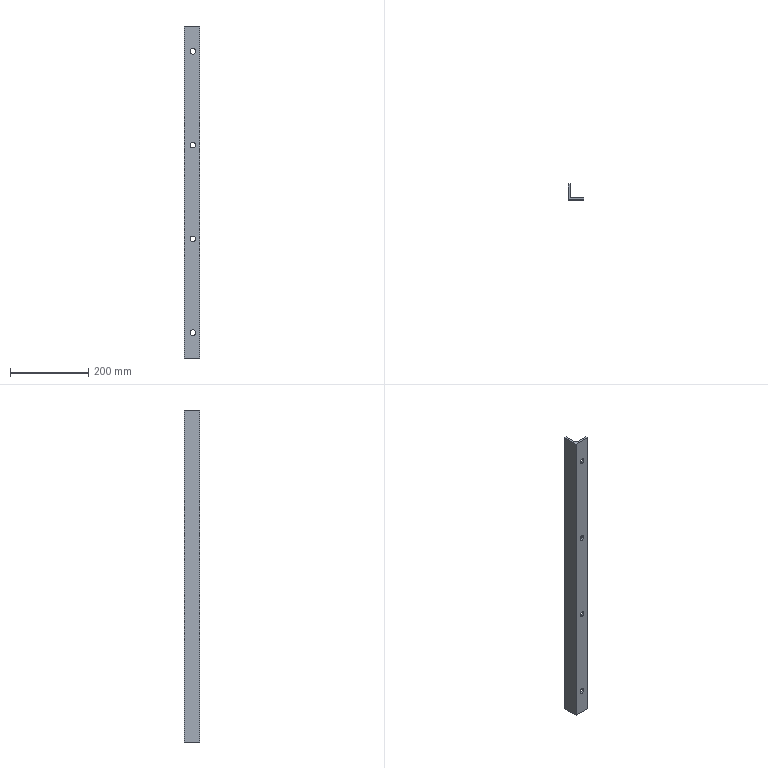Part | NX | features BREP 1 | 1 solid | 17 faces | box 40 x 40 x 850 mm | volume 320232 mm3 | cylinder 9 | plane 8 | commonest cylinder face diameters 14 x8 10 x1
STEP:
#1=CARTESIAN_POINT('',(22.,0.,353.));
#2=VERTEX_POINT('',#1);
#3=CARTESIAN_POINT('',(22.,0.,367.));
#4=VERTEX_POINT('',#3);
#5=CARTESIAN_POINT('',(22.,0.,360.));
#6=DIRECTION('',(0.,1.,0.));
#7=DIRECTION('',(0.,0.,-1.));
#8=AXIS2_PLACEMENT_3D('',#5,#6,#7);
#9=CIRCLE('',#8,7.);
#10=EDGE_CURVE('',#2,#4,#9,.T.);
#11=ORIENTED_EDGE('',*,*,#10,.F.);
#12=CARTESIAN_POINT('',(22.,5.,353.));
#13=VERTEX_POINT('',#12);
#14=CARTESIAN_POINT('',(22.,0.,353.));
#15=DIRECTION('',(0.,1.,0.));
#16=VECTOR('',#15,1000.);
#17=LINE('',#14,#16);
#18=EDGE_CURVE('',#2,#13,#17,.T.);
#19=ORIENTED_EDGE('',*,*,#18,.T.);
#20=CARTESIAN_POINT('',(22.,5.,367.));
#21=VERTEX_POINT('',#20);
#22=CARTESIAN_POINT('',(22.,5.,360.));
#23=DIRECTION('',(0.,1.,0.));
#24=DIRECTION('',(0.,0.,-1.));
#25=AXIS2_PLACEMENT_3D('',#22,#23,#24);
#26=CIRCLE('',#25,7.);
#27=EDGE_CURVE('',#13,#21,#26,.T.);
#28=ORIENTED_EDGE('',*,*,#27,.T.);
#29=CARTESIAN_POINT('',(22.,0.,367.));
#30=DIRECTION('',(0.,1.,0.));
#31=VECTOR('',#30,1000.);
#32=LINE('',#29,#31);
#33=EDGE_CURVE('',#4,#21,#32,.T.);
#34=ORIENTED_EDGE('',*,*,#33,.F.);
#35=EDGE_LOOP('',(#11,#19,#28,#34));
#36=FACE_BOUND('',#35,.T.);
#37=CARTESIAN_POINT('',(22.,0.,360.));
#38=DIRECTION('',(0.,1.,0.));
#39=DIRECTION('',(0.,0.,-1.));
#40=AXIS2_PLACEMENT_3D('',#37,#38,#39);
#41=CYLINDRICAL_SURFACE('',#40,7.);
#42=ADVANCED_FACE('',(#36),#41,.F.);
#43=CARTESIAN_POINT('',(22.,0.,113.));
#44=VERTEX_POINT('',#43);
#45=CARTESIAN_POINT('',(22.,0.,127.));
#46=VERTEX_POINT('',#45);
#47=CARTESIAN_POINT('',(22.,0.,120.));
#48=DIRECTION('',(0.,1.,0.));
#49=DIRECTION('',(0.,0.,-1.));
#50=AXIS2_PLACEMENT_3D('',#47,#48,#49);
#51=CIRCLE('',#50,7.);
#52=EDGE_CURVE('',#44,#46,#51,.T.);
#53=ORIENTED_EDGE('',*,*,#52,.F.);
#54=CARTESIAN_POINT('',(22.,5.,113.));
#55=VERTEX_POINT('',#54);
#56=CARTESIAN_POINT('',(22.,0.,113.));
#57=DIRECTION('',(0.,1.,0.));
#58=VECTOR('',#57,1000.);
#59=LINE('',#56,#58);
#60=EDGE_CURVE('',#44,#55,#59,.T.);
#61=ORIENTED_EDGE('',*,*,#60,.T.);
#62=CARTESIAN_POINT('',(22.,5.,127.));
#63=VERTEX_POINT('',#62);
#64=CARTESIAN_POINT('',(22.,5.,120.));
#65=DIRECTION('',(0.,1.,0.));
#66=DIRECTION('',(0.,0.,-1.));
#67=AXIS2_PLACEMENT_3D('',#64,#65,#66);
#68=CIRCLE('',#67,7.);
#69=EDGE_CURVE('',#55,#63,#68,.T.);
#70=ORIENTED_EDGE('',*,*,#69,.T.);
#71=CARTESIAN_POINT('',(22.,0.,127.));
#72=DIRECTION('',(0.,1.,0.));
#73=VECTOR('',#72,1000.);
#74=LINE('',#71,#73);
#75=EDGE_CURVE('',#46,#63,#74,.T.);
#76=ORIENTED_EDGE('',*,*,#75,.F.);
#77=EDGE_LOOP('',(#53,#61,#70,#76));
#78=FACE_BOUND('',#77,.T.);
#79=CARTESIAN_POINT('',(22.,0.,120.));
#80=DIRECTION('',(0.,1.,0.));
#81=DIRECTION('',(0.,0.,-1.));
#82=AXIS2_PLACEMENT_3D('',#79,#80,#81);
#83=CYLINDRICAL_SURFACE('',#82,7.);
#84=ADVANCED_FACE('',(#78),#83,.F.);
#85=CARTESIAN_POINT('',(22.,0.,-127.));
#86=VERTEX_POINT('',#85);
#87=CARTESIAN_POINT('',(22.,0.,-113.));
#88=VERTEX_POINT('',#87);
#89=CARTESIAN_POINT('',(22.,0.,-120.));
#90=DIRECTION('',(0.,1.,0.));
#91=DIRECTION('',(0.,0.,1.));
#92=AXIS2_PLACEMENT_3D('',#89,#90,#91);
#93=CIRCLE('',#92,7.);
#94=EDGE_CURVE('',#86,#88,#93,.T.);
#95=ORIENTED_EDGE('',*,*,#94,.F.);
#96=CARTESIAN_POINT('',(22.,5.,-127.));
#97=VERTEX_POINT('',#96);
#98=CARTESIAN_POINT('',(22.,0.,-127.));
#99=DIRECTION('',(0.,1.,0.));
#100=VECTOR('',#99,1000.);
#101=LINE('',#98,#100);
#102=EDGE_CURVE('',#86,#97,#101,.T.);
#103=ORIENTED_EDGE('',*,*,#102,.T.);
#104=CARTESIAN_POINT('',(22.,5.,-113.));
#105=VERTEX_POINT('',#104);
#106=CARTESIAN_POINT('',(22.,5.,-120.));
#107=DIRECTION('',(0.,1.,0.));
#108=DIRECTION('',(0.,0.,1.));
#109=AXIS2_PLACEMENT_3D('',#106,#107,#108);
#110=CIRCLE('',#109,7.);
#111=EDGE_CURVE('',#97,#105,#110,.T.);
#112=ORIENTED_EDGE('',*,*,#111,.T.);
#113=CARTESIAN_POINT('',(22.,0.,-113.));
#114=DIRECTION('',(0.,1.,0.));
#115=VECTOR('',#114,1000.);
#116=LINE('',#113,#115);
#117=EDGE_CURVE('',#88,#105,#116,.T.);
#118=ORIENTED_EDGE('',*,*,#117,.F.);
#119=EDGE_LOOP('',(#95,#103,#112,#118));
#120=FACE_BOUND('',#119,.T.);
#121=CARTESIAN_POINT('',(22.,0.,-120.));
#122=DIRECTION('',(0.,1.,0.));
#123=DIRECTION('',(0.,0.,-1.));
#124=AXIS2_PLACEMENT_3D('',#121,#122,#123);
#125=CYLINDRICAL_SURFACE('',#124,7.);
#126=ADVANCED_FACE('',(#120),#125,.F.);
#127=CARTESIAN_POINT('',(22.,0.,-367.));
#128=VERTEX_POINT('',#127);
#129=CARTESIAN_POINT('',(22.,0.,-353.));
#130=VERTEX_POINT('',#129);
#131=CARTESIAN_POINT('',(22.,0.,-360.));
#132=DIRECTION('',(0.,1.,0.));
#133=DIRECTION('',(0.,0.,1.));
#134=AXIS2_PLACEMENT_3D('',#131,#132,#133);
#135=CIRCLE('',#134,7.);
#136=EDGE_CURVE('',#128,#130,#135,.T.);
#137=ORIENTED_EDGE('',*,*,#136,.F.);
#138=CARTESIAN_POINT('',(22.,5.,-367.));
#139=VERTEX_POINT('',#138);
#140=CARTESIAN_POINT('',(22.,0.,-367.));
#141=DIRECTION('',(0.,1.,0.));
#142=VECTOR('',#141,1000.);
#143=LINE('',#140,#142);
#144=EDGE_CURVE('',#128,#139,#143,.T.);
#145=ORIENTED_EDGE('',*,*,#144,.T.);
#146=CARTESIAN_POINT('',(22.,5.,-353.));
#147=VERTEX_POINT('',#146);
#148=CARTESIAN_POINT('',(22.,5.,-360.));
#149=DIRECTION('',(0.,1.,0.));
#150=DIRECTION('',(0.,0.,1.));
#151=AXIS2_PLACEMENT_3D('',#148,#149,#150);
#152=CIRCLE('',#151,7.);
#153=EDGE_CURVE('',#139,#147,#152,.T.);
#154=ORIENTED_EDGE('',*,*,#153,.T.);
#155=CARTESIAN_POINT('',(22.,0.,-353.));
#156=DIRECTION('',(0.,1.,0.));
#157=VECTOR('',#156,1000.);
#158=LINE('',#155,#157);
#159=EDGE_CURVE('',#130,#147,#158,.T.);
#160=ORIENTED_EDGE('',*,*,#159,.F.);
#161=EDGE_LOOP('',(#137,#145,#154,#160));
#162=FACE_BOUND('',#161,.T.);
#163=CARTESIAN_POINT('',(22.,0.,-360.));
#164=DIRECTION('',(0.,1.,0.));
#165=DIRECTION('',(0.,0.,-1.));
#166=AXIS2_PLACEMENT_3D('',#163,#164,#165);
#167=CYLINDRICAL_SURFACE('',#166,7.);
#168=ADVANCED_FACE('',(#162),#167,.F.);
#169=CARTESIAN_POINT('',(40.,0.,-425.));
#170=VERTEX_POINT('',#169);
#171=CARTESIAN_POINT('',(40.,5.,-425.));
#172=VERTEX_POINT('',#171);
#173=CARTESIAN_POINT('',(40.,5.,-425.));
#174=DIRECTION('',(0.,1.,0.));
#175=VECTOR('',#174,1000.);
#176=LINE('',#173,#175);
#177=EDGE_CURVE('',#170,#172,#176,.T.);
#178=ORIENTED_EDGE('',*,*,#177,.T.);
#179=CARTESIAN_POINT('',(40.,5.,425.));
#180=VERTEX_POINT('',#179);
#181=CARTESIAN_POINT('',(40.,5.,425.));
#182=DIRECTION('',(0.,0.,-1.));
#183=VECTOR('',#182,1000.);
#184=LINE('',#181,#183);
#185=EDGE_CURVE('',#180,#172,#184,.T.);
#186=ORIENTED_EDGE('',*,*,#185,.F.);
#187=CARTESIAN_POINT('',(40.,0.,425.));
#188=VERTEX_POINT('',#187);
#189=CARTESIAN_POINT('',(40.,5.,425.));
#190=DIRECTION('',(0.,1.,0.));
#191=VECTOR('',#190,1000.);
#192=LINE('',#189,#191);
#193=EDGE_CURVE('',#188,#180,#192,.T.);
#194=ORIENTED_EDGE('',*,*,#193,.F.);
#195=CARTESIAN_POINT('',(40.,0.,425.));
#196=DIRECTION('',(0.,0.,-1.));
#197=VECTOR('',#196,1000.);
#198=LINE('',#195,#197);
#199=EDGE_CURVE('',#188,#170,#198,.T.);
#200=ORIENTED_EDGE('',*,*,#199,.T.);
#201=EDGE_LOOP('',(#178,#186,#194,#200));
#202=FACE_BOUND('',#201,.T.);
#203=CARTESIAN_POINT('',(40.,5.,425.));
#204=DIRECTION('',(-1.,0.,0.));
#205=DIRECTION('',(0.,0.,-1.));
#206=AXIS2_PLACEMENT_3D('',#203,#204,#205);
#207=PLANE('',#206);
#208=ADVANCED_FACE('',(#202),#207,.F.);
#209=CARTESIAN_POINT('',(22.,5.,360.));
#210=DIRECTION('',(0.,1.,0.));
#211=DIRECTION('',(0.,0.,-1.));
#212=AXIS2_PLACEMENT_3D('',#209,#210,#211);
#213=CIRCLE('',#212,7.);
#214=EDGE_CURVE('',#21,#13,#213,.T.);
#215=ORIENTED_EDGE('',*,*,#214,.F.);
#216=ORIENTED_EDGE('',*,*,#27,.F.);
#217=EDGE_LOOP('',(#215,#216));
#218=FACE_BOUND('',#217,.T.);
#219=CARTESIAN_POINT('',(22.,5.,120.));
#220=DIRECTION('',(0.,1.,0.));
#221=DIRECTION('',(0.,0.,-1.));
#222=AXIS2_PLACEMENT_3D('',#219,#220,#221);
#223=CIRCLE('',#222,7.);
#224=EDGE_CURVE('',#63,#55,#223,.T.);
#225=ORIENTED_EDGE('',*,*,#224,.F.);
#226=ORIENTED_EDGE('',*,*,#69,.F.);
#227=EDGE_LOOP('',(#225,#226));
#228=FACE_BOUND('',#227,.T.);
#229=CARTESIAN_POINT('',(22.,5.,-120.));
#230=DIRECTION('',(0.,1.,0.));
#231=DIRECTION('',(0.,0.,1.));
#232=AXIS2_PLACEMENT_3D('',#229,#230,#231);
#233=CIRCLE('',#232,7.);
#234=EDGE_CURVE('',#105,#97,#233,.T.);
#235=ORIENTED_EDGE('',*,*,#234,.F.);
#236=ORIENTED_EDGE('',*,*,#111,.F.);
#237=EDGE_LOOP('',(#235,#236));
#238=FACE_BOUND('',#237,.T.);
#239=CARTESIAN_POINT('',(22.,5.,-360.));
#240=DIRECTION('',(0.,1.,0.));
#241=DIRECTION('',(0.,0.,1.));
#242=AXIS2_PLACEMENT_3D('',#239,#240,#241);
#243=CIRCLE('',#242,7.);
#244=EDGE_CURVE('',#147,#139,#243,.T.);
#245=ORIENTED_EDGE('',*,*,#244,.F.);
#246=ORIENTED_EDGE('',*,*,#153,.F.);
#247=EDGE_LOOP('',(#245,#246));
#248=FACE_BOUND('',#247,.T.);
#249=CARTESIAN_POINT('',(10.,5.,-425.));
#250=VERTEX_POINT('',#249);
#251=CARTESIAN_POINT('',(10.,5.,-425.));
#252=DIRECTION('',(-1.,0.,0.));
#253=VECTOR('',#252,1000.);
#254=LINE('',#251,#253);
#255=EDGE_CURVE('',#172,#250,#254,.T.);
#256=ORIENTED_EDGE('',*,*,#255,.T.);
#257=CARTESIAN_POINT('',(10.,5.,425.));
#258=VERTEX_POINT('',#257);
#259=CARTESIAN_POINT('',(10.,5.,425.));
#260=DIRECTION('',(0.,0.,-1.));
#261=VECTOR('',#260,1000.);
#262=LINE('',#259,#261);
#263=EDGE_CURVE('',#258,#250,#262,.T.);
#264=ORIENTED_EDGE('',*,*,#263,.F.);
#265=CARTESIAN_POINT('',(10.,5.,425.));
#266=DIRECTION('',(-1.,0.,0.));
#267=VECTOR('',#266,1000.);
#268=LINE('',#265,#267);
#269=EDGE_CURVE('',#180,#258,#268,.T.);
#270=ORIENTED_EDGE('',*,*,#269,.F.);
#271=ORIENTED_EDGE('',*,*,#185,.T.);
#272=EDGE_LOOP('',(#256,#264,#270,#271));
#273=FACE_BOUND('',#272,.T.);
#274=CARTESIAN_POINT('',(10.,5.,425.));
#275=DIRECTION('',(0.,-1.,0.));
#276=DIRECTION('',(0.,0.,1.));
#277=AXIS2_PLACEMENT_3D('',#274,#275,#276);
#278=PLANE('',#277);
#279=ADVANCED_FACE('',(#218,#228,#238,#248,#273),#278,.F.);
#280=CARTESIAN_POINT('',(5.,10.,-425.));
#281=VERTEX_POINT('',#280);
#282=CARTESIAN_POINT('',(10.,10.,-425.));
#283=DIRECTION('',(0.,0.,-1.));
#284=DIRECTION('',(1.,0.,0.));
#285=AXIS2_PLACEMENT_3D('',#282,#283,#284);
#286=CIRCLE('',#285,5.);
#287=EDGE_CURVE('',#250,#281,#286,.T.);
#288=ORIENTED_EDGE('',*,*,#287,.T.);
#289=CARTESIAN_POINT('',(5.,10.,425.));
#290=VERTEX_POINT('',#289);
#291=CARTESIAN_POINT('',(5.,10.,425.));
#292=DIRECTION('',(0.,0.,-1.));
#293=VECTOR('',#292,1000.);
#294=LINE('',#291,#293);
#295=EDGE_CURVE('',#290,#281,#294,.T.);
#296=ORIENTED_EDGE('',*,*,#295,.F.);
#297=CARTESIAN_POINT('',(10.,10.,425.));
#298=DIRECTION('',(0.,0.,-1.));
#299=DIRECTION('',(1.,0.,0.));
#300=AXIS2_PLACEMENT_3D('',#297,#298,#299);
#301=CIRCLE('',#300,5.);
#302=EDGE_CURVE('',#258,#290,#301,.T.);
#303=ORIENTED_EDGE('',*,*,#302,.F.);
#304=ORIENTED_EDGE('',*,*,#263,.T.);
#305=EDGE_LOOP('',(#288,#296,#303,#304));
#306=FACE_BOUND('',#305,.T.);
#307=CARTESIAN_POINT('',(10.,10.,425.));
#308=DIRECTION('',(0.,0.,-1.));
#309=DIRECTION('',(1.,0.,0.));
#310=AXIS2_PLACEMENT_3D('',#307,#308,#309);
#311=CYLINDRICAL_SURFACE('',#310,5.);
#312=ADVANCED_FACE('',(#306),#311,.F.);
#313=CARTESIAN_POINT('',(5.,40.,-425.));
#314=VERTEX_POINT('',#313);
#315=CARTESIAN_POINT('',(5.,40.,-425.));
#316=DIRECTION('',(0.,1.,0.));
#317=VECTOR('',#316,1000.);
#318=LINE('',#315,#317);
#319=EDGE_CURVE('',#281,#314,#318,.T.);
#320=ORIENTED_EDGE('',*,*,#319,.T.);
#321=CARTESIAN_POINT('',(5.,40.,425.));
#322=VERTEX_POINT('',#321);
#323=CARTESIAN_POINT('',(5.,40.,425.));
#324=DIRECTION('',(0.,0.,-1.));
#325=VECTOR('',#324,1000.);
#326=LINE('',#323,#325);
#327=EDGE_CURVE('',#322,#314,#326,.T.);
#328=ORIENTED_EDGE('',*,*,#327,.F.);
#329=CARTESIAN_POINT('',(5.,40.,425.));
#330=DIRECTION('',(0.,1.,0.));
#331=VECTOR('',#330,1000.);
#332=LINE('',#329,#331);
#333=EDGE_CURVE('',#290,#322,#332,.T.);
#334=ORIENTED_EDGE('',*,*,#333,.F.);
#335=ORIENTED_EDGE('',*,*,#295,.T.);
#336=EDGE_LOOP('',(#320,#328,#334,#335));
#337=FACE_BOUND('',#336,.T.);
#338=CARTESIAN_POINT('',(5.,40.,425.));
#339=DIRECTION('',(-1.,0.,0.));
#340=DIRECTION('',(0.,0.,-1.));
#341=AXIS2_PLACEMENT_3D('',#338,#339,#340);
#342=PLANE('',#341);
#343=ADVANCED_FACE('',(#337),#342,.F.);
#344=CARTESIAN_POINT('',(0.,40.,-425.));
#345=VERTEX_POINT('',#344);
#346=CARTESIAN_POINT('',(0.,40.,-425.));
#347=DIRECTION('',(-1.,0.,0.));
#348=VECTOR('',#347,1000.);
#349=LINE('',#346,#348);
#350=EDGE_CURVE('',#314,#345,#349,.T.);
#351=ORIENTED_EDGE('',*,*,#350,.T.);
#352=CARTESIAN_POINT('',(0.,40.,425.));
#353=VERTEX_POINT('',#352);
#354=CARTESIAN_POINT('',(0.,40.,425.));
#355=DIRECTION('',(0.,0.,-1.));
#356=VECTOR('',#355,1000.);
#357=LINE('',#354,#356);
#358=EDGE_CURVE('',#353,#345,#357,.T.);
#359=ORIENTED_EDGE('',*,*,#358,.F.);
#360=CARTESIAN_POINT('',(0.,40.,425.));
#361=DIRECTION('',(-1.,0.,0.));
#362=VECTOR('',#361,1000.);
#363=LINE('',#360,#362);
#364=EDGE_CURVE('',#322,#353,#363,.T.);
#365=ORIENTED_EDGE('',*,*,#364,.F.);
#366=ORIENTED_EDGE('',*,*,#327,.T.);
#367=EDGE_LOOP('',(#351,#359,#365,#366));
#368=FACE_BOUND('',#367,.T.);
#369=CARTESIAN_POINT('',(0.,40.,425.));
#370=DIRECTION('',(0.,-1.,0.));
#371=DIRECTION('',(0.,0.,1.));
#372=AXIS2_PLACEMENT_3D('',#369,#370,#371);
#373=PLANE('',#372);
#374=ADVANCED_FACE('',(#368),#373,.F.);
#375=CARTESIAN_POINT('',(0.,0.,-425.));
#376=VERTEX_POINT('',#375);
#377=CARTESIAN_POINT('',(0.,0.,-425.));
#378=DIRECTION('',(0.,-1.,0.));
#379=VECTOR('',#378,1000.);
#380=LINE('',#377,#379);
#381=EDGE_CURVE('',#345,#376,#380,.T.);
#382=ORIENTED_EDGE('',*,*,#381,.T.);
#383=CARTESIAN_POINT('',(0.,0.,425.));
#384=VERTEX_POINT('',#383);
#385=CARTESIAN_POINT('',(0.,0.,425.));
#386=DIRECTION('',(0.,0.,-1.));
#387=VECTOR('',#386,1000.);
#388=LINE('',#385,#387);
#389=EDGE_CURVE('',#384,#376,#388,.T.);
#390=ORIENTED_EDGE('',*,*,#389,.F.);
#391=CARTESIAN_POINT('',(0.,0.,425.));
#392=DIRECTION('',(0.,-1.,0.));
#393=VECTOR('',#392,1000.);
#394=LINE('',#391,#393);
#395=EDGE_CURVE('',#353,#384,#394,.T.);
#396=ORIENTED_EDGE('',*,*,#395,.F.);
#397=ORIENTED_EDGE('',*,*,#358,.T.);
#398=EDGE_LOOP('',(#382,#390,#396,#397));
#399=FACE_BOUND('',#398,.T.);
#400=CARTESIAN_POINT('',(0.,0.,425.));
#401=DIRECTION('',(1.,0.,0.));
#402=DIRECTION('',(0.,0.,1.));
#403=AXIS2_PLACEMENT_3D('',#400,#401,#402);
#404=PLANE('',#403);
#405=ADVANCED_FACE('',(#399),#404,.F.);
#406=CARTESIAN_POINT('',(22.,0.,360.));
#407=DIRECTION('',(0.,1.,0.));
#408=DIRECTION('',(0.,0.,-1.));
#409=AXIS2_PLACEMENT_3D('',#406,#407,#408);
#410=CIRCLE('',#409,7.);
#411=EDGE_CURVE('',#4,#2,#410,.T.);
#412=ORIENTED_EDGE('',*,*,#411,.T.);
#413=ORIENTED_EDGE('',*,*,#10,.T.);
#414=EDGE_LOOP('',(#412,#413));
#415=FACE_BOUND('',#414,.T.);
#416=CARTESIAN_POINT('',(22.,0.,120.));
#417=DIRECTION('',(0.,1.,0.));
#418=DIRECTION('',(0.,0.,-1.));
#419=AXIS2_PLACEMENT_3D('',#416,#417,#418);
#420=CIRCLE('',#419,7.);
#421=EDGE_CURVE('',#46,#44,#420,.T.);
#422=ORIENTED_EDGE('',*,*,#421,.T.);
#423=ORIENTED_EDGE('',*,*,#52,.T.);
#424=EDGE_LOOP('',(#422,#423));
#425=FACE_BOUND('',#424,.T.);
#426=CARTESIAN_POINT('',(22.,0.,-120.));
#427=DIRECTION('',(0.,1.,0.));
#428=DIRECTION('',(0.,0.,1.));
#429=AXIS2_PLACEMENT_3D('',#426,#427,#428);
#430=CIRCLE('',#429,7.);
#431=EDGE_CURVE('',#88,#86,#430,.T.);
#432=ORIENTED_EDGE('',*,*,#431,.T.);
#433=ORIENTED_EDGE('',*,*,#94,.T.);
#434=EDGE_LOOP('',(#432,#433));
#435=FACE_BOUND('',#434,.T.);
#436=CARTESIAN_POINT('',(22.,0.,-360.));
#437=DIRECTION('',(0.,1.,0.));
#438=DIRECTION('',(0.,0.,1.));
#439=AXIS2_PLACEMENT_3D('',#436,#437,#438);
#440=CIRCLE('',#439,7.);
#441=EDGE_CURVE('',#130,#128,#440,.T.);
#442=ORIENTED_EDGE('',*,*,#441,.T.);
#443=ORIENTED_EDGE('',*,*,#136,.T.);
#444=EDGE_LOOP('',(#442,#443));
#445=FACE_BOUND('',#444,.T.);
#446=CARTESIAN_POINT('',(40.,0.,-425.));
#447=DIRECTION('',(1.,0.,0.));
#448=VECTOR('',#447,1000.);
#449=LINE('',#446,#448);
#450=EDGE_CURVE('',#376,#170,#449,.T.);
#451=ORIENTED_EDGE('',*,*,#450,.T.);
#452=ORIENTED_EDGE('',*,*,#199,.F.);
#453=CARTESIAN_POINT('',(40.,0.,425.));
#454=DIRECTION('',(1.,0.,0.));
#455=VECTOR('',#454,1000.);
#456=LINE('',#453,#455);
#457=EDGE_CURVE('',#384,#188,#456,.T.);
#458=ORIENTED_EDGE('',*,*,#457,.F.);
#459=ORIENTED_EDGE('',*,*,#389,.T.);
#460=EDGE_LOOP('',(#451,#452,#458,#459));
#461=FACE_BOUND('',#460,.T.);
#462=CARTESIAN_POINT('',(40.,0.,425.));
#463=DIRECTION('',(0.,1.,0.));
#464=DIRECTION('',(0.,0.,-1.));
#465=AXIS2_PLACEMENT_3D('',#462,#463,#464);
#466=PLANE('',#465);
#467=ADVANCED_FACE('',(#415,#425,#435,#445,#461),#466,.F.);
#468=ORIENTED_EDGE('',*,*,#193,.T.);
#469=ORIENTED_EDGE('',*,*,#269,.T.);
#470=ORIENTED_EDGE('',*,*,#302,.T.);
#471=ORIENTED_EDGE('',*,*,#333,.T.);
#472=ORIENTED_EDGE('',*,*,#364,.T.);
#473=ORIENTED_EDGE('',*,*,#395,.T.);
#474=ORIENTED_EDGE('',*,*,#457,.T.);
#475=EDGE_LOOP('',(#468,#469,#470,#471,#472,#473,#474));
#476=FACE_BOUND('',#475,.T.);
#477=CARTESIAN_POINT('',(10.,10.,425.));
#478=DIRECTION('',(0.,0.,1.));
#479=DIRECTION('',(-1.,0.,0.));
#480=AXIS2_PLACEMENT_3D('',#477,#478,#479);
#481=PLANE('',#480);
#482=ADVANCED_FACE('',(#476),#481,.T.);
#483=ORIENTED_EDGE('',*,*,#177,.F.);
#484=ORIENTED_EDGE('',*,*,#450,.F.);
#485=ORIENTED_EDGE('',*,*,#381,.F.);
#486=ORIENTED_EDGE('',*,*,#350,.F.);
#487=ORIENTED_EDGE('',*,*,#319,.F.);
#488=ORIENTED_EDGE('',*,*,#287,.F.);
#489=ORIENTED_EDGE('',*,*,#255,.F.);
#490=EDGE_LOOP('',(#483,#484,#485,#486,#487,#488,#489));
#491=FACE_BOUND('',#490,.T.);
#492=CARTESIAN_POINT('',(10.,10.,-425.));
#493=DIRECTION('',(0.,0.,1.));
#494=DIRECTION('',(-1.,0.,0.));
#495=AXIS2_PLACEMENT_3D('',#492,#493,#494);
#496=PLANE('',#495);
#497=ADVANCED_FACE('',(#491),#496,.F.);
#498=ORIENTED_EDGE('',*,*,#144,.F.);
#499=ORIENTED_EDGE('',*,*,#441,.F.);
#500=ORIENTED_EDGE('',*,*,#159,.T.);
#501=ORIENTED_EDGE('',*,*,#244,.T.);
#502=EDGE_LOOP('',(#498,#499,#500,#501));
#503=FACE_BOUND('',#502,.T.);
#504=CARTESIAN_POINT('',(22.,0.,-360.));
#505=DIRECTION('',(0.,1.,0.));
#506=DIRECTION('',(0.,0.,-1.));
#507=AXIS2_PLACEMENT_3D('',#504,#505,#506);
#508=CYLINDRICAL_SURFACE('',#507,7.);
#509=ADVANCED_FACE('',(#503),#508,.F.);
#510=ORIENTED_EDGE('',*,*,#102,.F.);
#511=ORIENTED_EDGE('',*,*,#431,.F.);
#512=ORIENTED_EDGE('',*,*,#117,.T.);
#513=ORIENTED_EDGE('',*,*,#234,.T.);
#514=EDGE_LOOP('',(#510,#511,#512,#513));
#515=FACE_BOUND('',#514,.T.);
#516=CARTESIAN_POINT('',(22.,0.,-120.));
#517=DIRECTION('',(0.,1.,0.));
#518=DIRECTION('',(0.,0.,-1.));
#519=AXIS2_PLACEMENT_3D('',#516,#517,#518);
#520=CYLINDRICAL_SURFACE('',#519,7.);
#521=ADVANCED_FACE('',(#515),#520,.F.);
#522=ORIENTED_EDGE('',*,*,#60,.F.);
#523=ORIENTED_EDGE('',*,*,#421,.F.);
#524=ORIENTED_EDGE('',*,*,#75,.T.);
#525=ORIENTED_EDGE('',*,*,#224,.T.);
#526=EDGE_LOOP('',(#522,#523,#524,#525));
#527=FACE_BOUND('',#526,.T.);
#528=CARTESIAN_POINT('',(22.,0.,120.));
#529=DIRECTION('',(0.,1.,0.));
#530=DIRECTION('',(0.,0.,-1.));
#531=AXIS2_PLACEMENT_3D('',#528,#529,#530);
#532=CYLINDRICAL_SURFACE('',#531,7.);
#533=ADVANCED_FACE('',(#527),#532,.F.);
#534=ORIENTED_EDGE('',*,*,#18,.F.);
#535=ORIENTED_EDGE('',*,*,#411,.F.);
#536=ORIENTED_EDGE('',*,*,#33,.T.);
#537=ORIENTED_EDGE('',*,*,#214,.T.);
#538=EDGE_LOOP('',(#534,#535,#536,#537));
#539=FACE_BOUND('',#538,.T.);
#540=CARTESIAN_POINT('',(22.,0.,360.));
#541=DIRECTION('',(0.,1.,0.));
#542=DIRECTION('',(0.,0.,-1.));
#543=AXIS2_PLACEMENT_3D('',#540,#541,#542);
#544=CYLINDRICAL_SURFACE('',#543,7.);
#545=ADVANCED_FACE('',(#539),#544,.F.);
#546=CLOSED_SHELL('',(#42,#84,#126,#168,#208,#279,#312,#343,#374,#405,#467,#482,#497,#509,#521,#533,#545));
#547=MANIFOLD_SOLID_BREP('',#546);
#548=(LENGTH_UNIT()NAMED_UNIT(*)SI_UNIT(.MILLI.,.METRE.));
#549=UNCERTAINTY_MEASURE_WITH_UNIT(LENGTH_MEASURE(0.00001),#548,'','');
#550=(NAMED_UNIT(*)PLANE_ANGLE_UNIT()SI_UNIT($,.RADIAN.));
#551=(NAMED_UNIT(*)SI_UNIT($,.STERADIAN.)SOLID_ANGLE_UNIT());
#552=(GEOMETRIC_REPRESENTATION_CONTEXT(3)GLOBAL_UNCERTAINTY_ASSIGNED_CONTEXT((#549))GLOBAL_UNIT_ASSIGNED_CONTEXT((#548,#550,#551))REPRESENTATION_CONTEXT('',''));
#553=ADVANCED_BREP_SHAPE_REPRESENTATION('',(#547),#552);